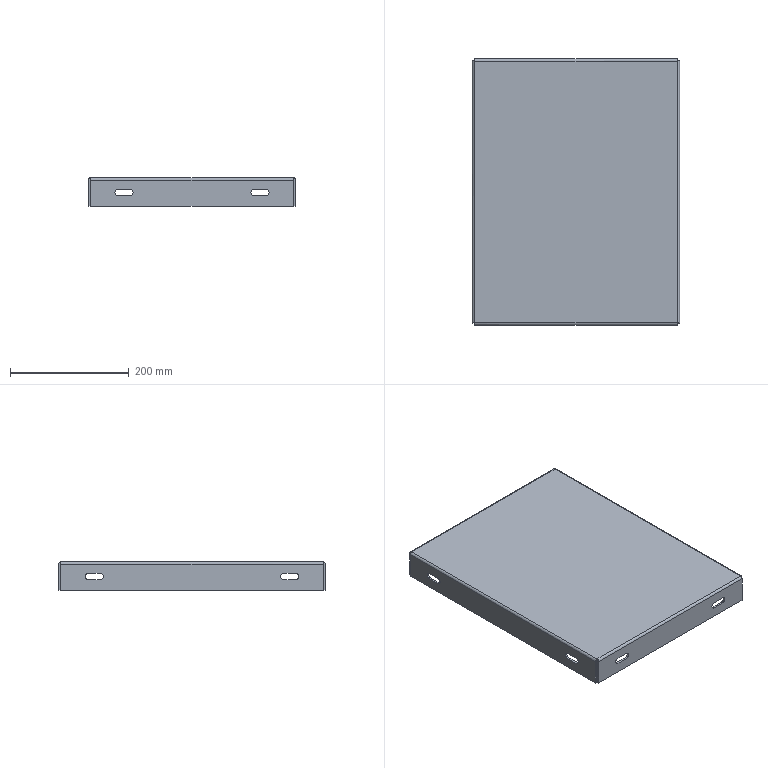Part | NX | features BREP 1 | 1 solid | 70 faces | box 349 x 449 x 48 mm | volume 669221 mm3 | plane 38 | cylinder 24 | spline 8 | commonest cylinder face diameters 10.5 x16 2 x4 8 x4